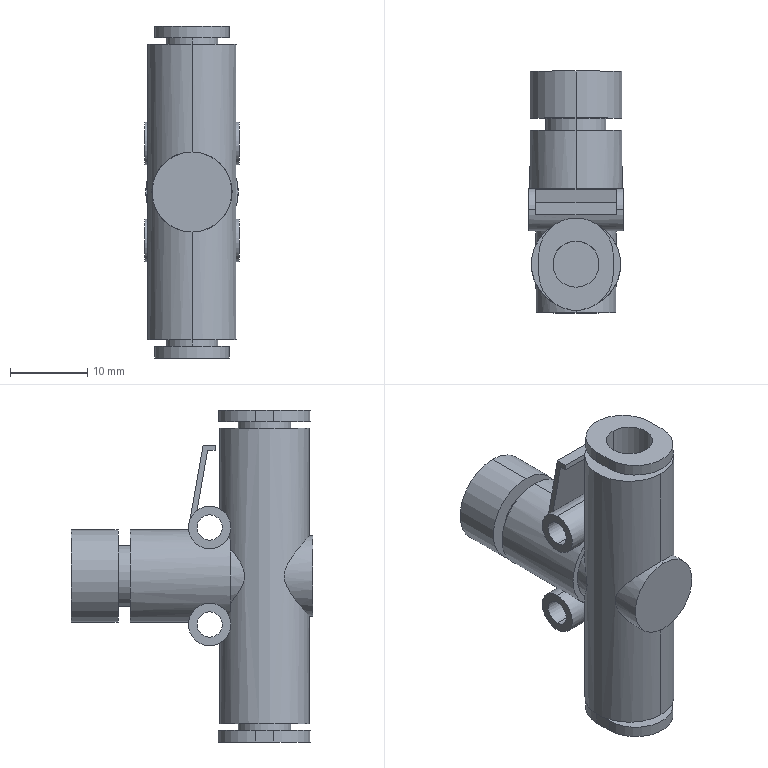Part | STEP file | AS2002FG-06A | 1 solid | 61 faces | box 12.3 x 31.4 x 43.1 mm | volume 6190 mm3 | cylinder 32 | plane 29 | commonest cylinder face diameters 3.3 x4 5.5 x4 6 x4 6.79 x4 9.7 x4 10.4 x4